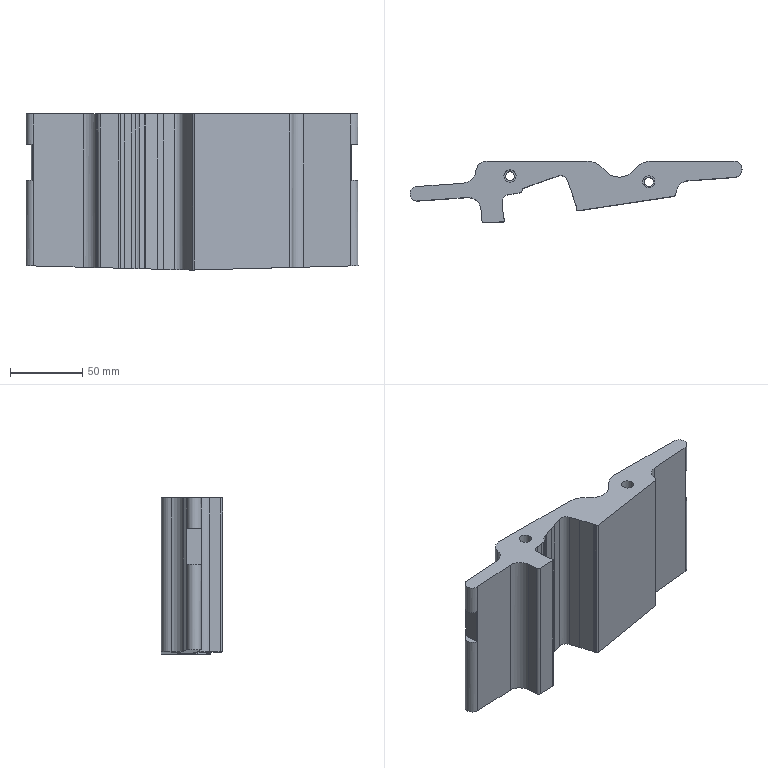Part | NX | features 8 2 | 1 solid | 57 faces | box 229.659 x 42.553 x 108 mm | volume 459816 mm3 | plane 32 | cylinder 25 | commonest cylinder face diameters 2 x6 4 x2 6.2 x2 8.5 x2 10 x2 30 x2